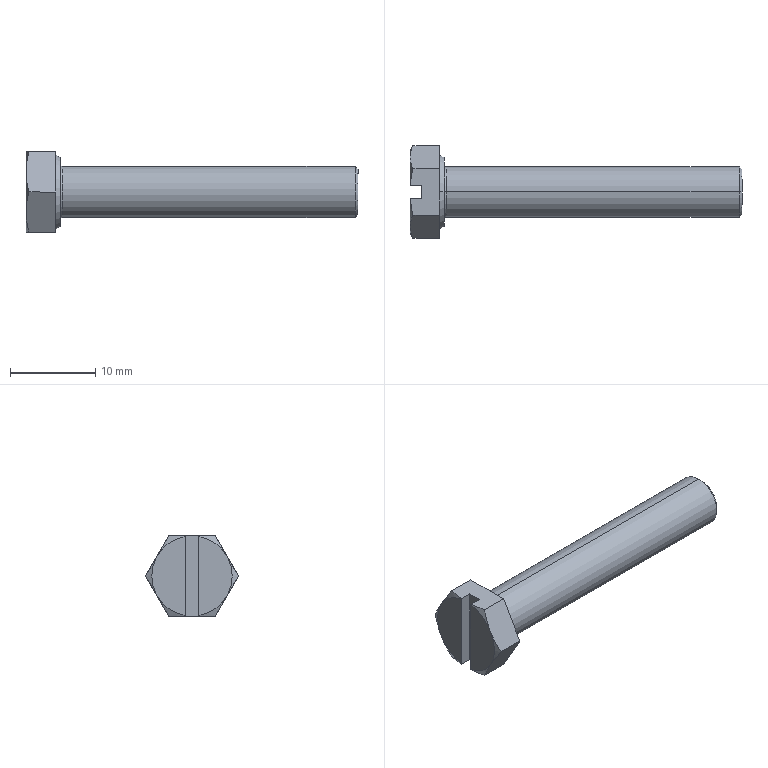Part | SolidWorks | features Cut 2, Chamfer 1, Extrusion 1, Fillet 1, LPattern 1, MoveCopyBody 1, RevCut 1, Revolution 1 | 1 solid | 24 faces | box 39 x 10.9 x 9.44 mm | volume 1265 mm3 | plane 14 | cone 6 | torus 2 | cylinder 2 | commonest cylinder face diameters 6 x2
STEP:
#1=CARTESIAN_POINT('',(28.65,0.,-9.517));
#2=VERTEX_POINT('',#1);
#3=CARTESIAN_POINT('',(28.65,0.,-4.183));
#4=VERTEX_POINT('',#3);
#5=CARTESIAN_POINT('',(28.65,0.,-6.85));
#6=DIRECTION('',(1.,0.,0.));
#7=DIRECTION('',(0.,0.,1.));
#8=AXIS2_PLACEMENT_3D('',#5,#6,#7);
#9=CIRCLE('',#8,2.667);
#10=EDGE_CURVE('',#2,#4,#9,.T.);
#11=ORIENTED_EDGE('',*,*,#10,.F.);
#12=CARTESIAN_POINT('',(28.317,0.,-9.85));
#13=VERTEX_POINT('',#12);
#14=CARTESIAN_POINT('',(28.317,0.,-9.85));
#15=DIRECTION('',(-0.7071,0.,-0.7071));
#16=VECTOR('',#15,1000.);
#17=LINE('',#14,#16);
#18=EDGE_CURVE('',#2,#13,#17,.T.);
#19=ORIENTED_EDGE('',*,*,#18,.T.);
#20=CARTESIAN_POINT('',(28.317,0.,-3.85));
#21=VERTEX_POINT('',#20);
#22=CARTESIAN_POINT('',(28.317,0.,-6.85));
#23=DIRECTION('',(-1.,0.,0.));
#24=DIRECTION('',(0.,0.,1.));
#25=AXIS2_PLACEMENT_3D('',#22,#23,#24);
#26=CIRCLE('',#25,3.);
#27=EDGE_CURVE('',#21,#13,#26,.T.);
#28=ORIENTED_EDGE('',*,*,#27,.F.);
#29=CARTESIAN_POINT('',(28.317,0.,-3.85));
#30=DIRECTION('',(-0.7071,0.,0.7071));
#31=VECTOR('',#30,1000.);
#32=LINE('',#29,#31);
#33=EDGE_CURVE('',#4,#21,#32,.T.);
#34=ORIENTED_EDGE('',*,*,#33,.F.);
#35=EDGE_LOOP('',(#11,#19,#28,#34));
#36=FACE_OUTER_BOUND('',#35,.T.);
#37=CARTESIAN_POINT('',(28.317,0.,-6.85));
#38=DIRECTION('',(-1.,0.,0.));
#39=DIRECTION('',(0.,0.,1.));
#40=AXIS2_PLACEMENT_3D('',#37,#38,#39);
#41=CONICAL_SURFACE('',#40,3.,0.7854);
#42=ADVANCED_FACE('',(#36),#41,.T.);
#43=CARTESIAN_POINT('',(-6.35,0.,-10.1));
#44=VERTEX_POINT('',#43);
#45=CARTESIAN_POINT('',(-6.35,0.,-3.6));
#46=VERTEX_POINT('',#45);
#47=CARTESIAN_POINT('',(-6.35,0.,-6.85));
#48=DIRECTION('',(-1.,0.,0.));
#49=DIRECTION('',(0.,0.,1.));
#50=AXIS2_PLACEMENT_3D('',#47,#48,#49);
#51=CIRCLE('',#50,3.25);
#52=EDGE_CURVE('',#44,#46,#51,.T.);
#53=ORIENTED_EDGE('',*,*,#52,.F.);
#54=CARTESIAN_POINT('',(-6.1,0.,-9.85));
#55=VERTEX_POINT('',#54);
#56=CARTESIAN_POINT('',(-6.1,0.,-10.1));
#57=DIRECTION('',(0.,1.,0.));
#58=DIRECTION('',(0.,0.,1.));
#59=AXIS2_PLACEMENT_3D('',#56,#57,#58);
#60=CIRCLE('',#59,0.25);
#61=EDGE_CURVE('',#44,#55,#60,.T.);
#62=ORIENTED_EDGE('',*,*,#61,.T.);
#63=CARTESIAN_POINT('',(-6.1,0.,-3.85));
#64=VERTEX_POINT('',#63);
#65=CARTESIAN_POINT('',(-6.1,0.,-6.85));
#66=DIRECTION('',(1.,0.,0.));
#67=DIRECTION('',(0.,0.,1.));
#68=AXIS2_PLACEMENT_3D('',#65,#66,#67);
#69=CIRCLE('',#68,3.);
#70=EDGE_CURVE('',#64,#55,#69,.T.);
#71=ORIENTED_EDGE('',*,*,#70,.F.);
#72=CARTESIAN_POINT('',(-6.1,0.,-3.6));
#73=DIRECTION('',(0.,-1.,0.));
#74=DIRECTION('',(0.,0.,-1.));
#75=AXIS2_PLACEMENT_3D('',#72,#73,#74);
#76=CIRCLE('',#75,0.25);
#77=EDGE_CURVE('',#46,#64,#76,.T.);
#78=ORIENTED_EDGE('',*,*,#77,.F.);
#79=EDGE_LOOP('',(#53,#62,#71,#78));
#80=FACE_OUTER_BOUND('',#79,.T.);
#81=CARTESIAN_POINT('',(-6.1,0.,-6.85));
#82=DIRECTION('',(-1.,0.,0.));
#83=DIRECTION('',(0.,0.,1.));
#84=AXIS2_PLACEMENT_3D('',#81,#82,#83);
#85=TOROIDAL_SURFACE('',#84,3.25,0.25);
#86=ADVANCED_FACE('',(#80),#85,.F.);
#87=CARTESIAN_POINT('',(-6.35,0.,-2.789));
#88=VERTEX_POINT('',#87);
#89=CARTESIAN_POINT('',(-6.35,0.,-10.911));
#90=VERTEX_POINT('',#89);
#91=CARTESIAN_POINT('',(-6.35,0.,-6.85));
#92=DIRECTION('',(-1.,0.,0.));
#93=DIRECTION('',(0.,0.,1.));
#94=AXIS2_PLACEMENT_3D('',#91,#92,#93);
#95=CIRCLE('',#94,4.061);
#96=EDGE_CURVE('',#88,#90,#95,.T.);
#97=ORIENTED_EDGE('',*,*,#96,.T.);
#98=CARTESIAN_POINT('',(-6.85,0.,-11.2));
#99=VERTEX_POINT('',#98);
#100=CARTESIAN_POINT('',(-6.35,0.,-10.911));
#101=DIRECTION('',(-0.866,0.,-0.5));
#102=VECTOR('',#101,1000.);
#103=LINE('',#100,#102);
#104=EDGE_CURVE('',#90,#99,#103,.T.);
#105=ORIENTED_EDGE('',*,*,#104,.T.);
#106=CARTESIAN_POINT('',(-6.85,0.,-2.5));
#107=VERTEX_POINT('',#106);
#108=CARTESIAN_POINT('',(-6.85,0.,-6.85));
#109=DIRECTION('',(1.,0.,0.));
#110=DIRECTION('',(0.,0.,1.));
#111=AXIS2_PLACEMENT_3D('',#108,#109,#110);
#112=CIRCLE('',#111,4.35);
#113=EDGE_CURVE('',#99,#107,#112,.T.);
#114=ORIENTED_EDGE('',*,*,#113,.T.);
#115=CARTESIAN_POINT('',(-6.35,0.,-2.789));
#116=DIRECTION('',(-0.866,0.,0.5));
#117=VECTOR('',#116,1000.);
#118=LINE('',#115,#117);
#119=EDGE_CURVE('',#88,#107,#118,.T.);
#120=ORIENTED_EDGE('',*,*,#119,.F.);
#121=EDGE_LOOP('',(#97,#105,#114,#120));
#122=FACE_OUTER_BOUND('',#121,.T.);
#123=CARTESIAN_POINT('',(-6.35,0.,-6.85));
#124=DIRECTION('',(-1.,0.,0.));
#125=DIRECTION('',(0.,0.,1.));
#126=AXIS2_PLACEMENT_3D('',#123,#124,#125);
#127=CONICAL_SURFACE('',#126,4.061,0.5236);
#128=ADVANCED_FACE('',(#122),#127,.T.);
#129=ORIENTED_EDGE('',*,*,#27,.T.);
#130=CARTESIAN_POINT('',(-6.85,0.,-9.85));
#131=DIRECTION('',(-1.,0.,0.));
#132=VECTOR('',#131,1000.);
#133=LINE('',#130,#132);
#134=EDGE_CURVE('',#13,#55,#133,.T.);
#135=ORIENTED_EDGE('',*,*,#134,.T.);
#136=CARTESIAN_POINT('',(-6.1,0.,-6.85));
#137=DIRECTION('',(1.,0.,0.));
#138=DIRECTION('',(0.,0.,1.));
#139=AXIS2_PLACEMENT_3D('',#136,#137,#138);
#140=CIRCLE('',#139,3.);
#141=EDGE_CURVE('',#55,#64,#140,.T.);
#142=ORIENTED_EDGE('',*,*,#141,.T.);
#143=CARTESIAN_POINT('',(-6.85,0.,-3.85));
#144=DIRECTION('',(-1.,0.,0.));
#145=VECTOR('',#144,1000.);
#146=LINE('',#143,#145);
#147=EDGE_CURVE('',#21,#64,#146,.T.);
#148=ORIENTED_EDGE('',*,*,#147,.F.);
#149=EDGE_LOOP('',(#129,#135,#142,#148));
#150=FACE_OUTER_BOUND('',#149,.T.);
#151=CARTESIAN_POINT('',(-6.85,0.,-6.85));
#152=DIRECTION('',(-1.,0.,0.));
#153=DIRECTION('',(0.,0.,1.));
#154=AXIS2_PLACEMENT_3D('',#151,#152,#153);
#155=CYLINDRICAL_SURFACE('',#154,3.);
#156=ADVANCED_FACE('',(#150),#155,.T.);
#157=CARTESIAN_POINT('',(-10.319,-0.8,-11.57));
#158=VERTEX_POINT('',#157);
#159=CARTESIAN_POINT('',(-10.35,-0.8,-11.501));
#160=VERTEX_POINT('',#159);
#161=CARTESIAN_POINT('',(-10.319,-0.8,-11.57));
#162=CARTESIAN_POINT('',(-10.329,-0.8,-11.547));
#163=CARTESIAN_POINT('',(-10.34,-0.8,-11.524));
#164=CARTESIAN_POINT('',(-10.35,-0.8,-11.501));
#165=B_SPLINE_CURVE_WITH_KNOTS('',3,(#161,#162,#163,#164),.UNSPECIFIED.,.F.,.F.,(4,4),(0.006283,0.006358),.UNSPECIFIED.);
#166=EDGE_CURVE('',#158,#160,#165,.T.);
#167=ORIENTED_EDGE('',*,*,#166,.F.);
#168=CARTESIAN_POINT('',(-10.009,-2.725,-11.57));
#169=VERTEX_POINT('',#168);
#170=CARTESIAN_POINT('',(-10.319,-0.8,-11.57));
#171=CARTESIAN_POINT('',(-10.293,-1.122,-11.57));
#172=CARTESIAN_POINT('',(-10.254,-1.444,-11.57));
#173=CARTESIAN_POINT('',(-10.149,-2.086,-11.57));
#174=CARTESIAN_POINT('',(-10.083,-2.408,-11.57));
#175=CARTESIAN_POINT('',(-10.009,-2.725,-11.57));
#176=B_SPLINE_CURVE_WITH_KNOTS('',3,(#170,#171,#172,#173,#174,#175),.UNSPECIFIED.,.F.,.F.,(4,2,4),(0.01518,0.01614,0.0171),.UNSPECIFIED.);
#177=EDGE_CURVE('',#158,#169,#176,.T.);
#178=ORIENTED_EDGE('',*,*,#177,.T.);
#179=CARTESIAN_POINT('',(-10.009,-5.45,-6.85));
#180=VERTEX_POINT('',#179);
#181=CARTESIAN_POINT('',(-10.009,-2.725,-11.57));
#182=CARTESIAN_POINT('',(-10.219,-3.174,-10.792));
#183=CARTESIAN_POINT('',(-10.349,-3.626,-10.01));
#184=CARTESIAN_POINT('',(-10.35,-4.309,-8.826));
#185=CARTESIAN_POINT('',(-10.32,-4.539,-8.428));
#186=CARTESIAN_POINT('',(-10.201,-4.998,-7.633));
#187=CARTESIAN_POINT('',(-10.115,-5.225,-7.24));
#188=CARTESIAN_POINT('',(-10.009,-5.45,-6.85));
#189=B_SPLINE_CURVE_WITH_KNOTS('',3,(#181,#182,#183,#184,#185,#186,#187,#188),.UNSPECIFIED.,.F.,.F.,(4,2,2,4),(0.000000234,0.00273,0.004094,0.005459),.UNSPECIFIED.);
#190=EDGE_CURVE('',#169,#180,#189,.T.);
#191=ORIENTED_EDGE('',*,*,#190,.T.);
#192=CARTESIAN_POINT('',(-10.009,-2.725,-2.13));
#193=VERTEX_POINT('',#192);
#194=CARTESIAN_POINT('',(-10.009,-5.45,-6.85));
#195=CARTESIAN_POINT('',(-10.219,-5.001,-6.072));
#196=CARTESIAN_POINT('',(-10.349,-4.549,-5.29));
#197=CARTESIAN_POINT('',(-10.35,-3.866,-4.106));
#198=CARTESIAN_POINT('',(-10.32,-3.636,-3.708));
#199=CARTESIAN_POINT('',(-10.201,-3.177,-2.914));
#200=CARTESIAN_POINT('',(-10.115,-2.95,-2.52));
#201=CARTESIAN_POINT('',(-10.009,-2.725,-2.13));
#202=B_SPLINE_CURVE_WITH_KNOTS('',3,(#194,#195,#196,#197,#198,#199,#200,#201),.UNSPECIFIED.,.F.,.F.,(4,2,2,4),(0.000000234,0.00273,0.004094,0.005459),.UNSPECIFIED.);
#203=EDGE_CURVE('',#180,#193,#202,.T.);
#204=ORIENTED_EDGE('',*,*,#203,.T.);
#205=CARTESIAN_POINT('',(-10.319,-0.8,-2.13));
#206=VERTEX_POINT('',#205);
#207=CARTESIAN_POINT('',(-10.009,-2.725,-2.13));
#208=CARTESIAN_POINT('',(-10.083,-2.408,-2.13));
#209=CARTESIAN_POINT('',(-10.149,-2.086,-2.13));
#210=CARTESIAN_POINT('',(-10.254,-1.444,-2.13));
#211=CARTESIAN_POINT('',(-10.293,-1.122,-2.13));
#212=CARTESIAN_POINT('',(-10.319,-0.8,-2.13));
#213=B_SPLINE_CURVE_WITH_KNOTS('',3,(#207,#208,#209,#210,#211,#212),.UNSPECIFIED.,.F.,.F.,(4,2,4),(0.004915,0.00589,0.006864),.UNSPECIFIED.);
#214=EDGE_CURVE('',#193,#206,#213,.T.);
#215=ORIENTED_EDGE('',*,*,#214,.T.);
#216=CARTESIAN_POINT('',(-10.35,-0.8,-2.199));
#217=VERTEX_POINT('',#216);
#218=CARTESIAN_POINT('',(-10.35,-0.8,-2.199));
#219=CARTESIAN_POINT('',(-10.34,-0.8,-2.176));
#220=CARTESIAN_POINT('',(-10.329,-0.8,-2.153));
#221=CARTESIAN_POINT('',(-10.319,-0.8,-2.13));
#222=B_SPLINE_CURVE_WITH_KNOTS('',3,(#218,#219,#220,#221),.UNSPECIFIED.,.F.,.F.,(4,4),(0.01639,0.01646),.UNSPECIFIED.);
#223=EDGE_CURVE('',#217,#206,#222,.T.);
#224=ORIENTED_EDGE('',*,*,#223,.F.);
#225=CARTESIAN_POINT('',(-10.35,0.,-6.85));
#226=DIRECTION('',(-1.,0.,0.));
#227=DIRECTION('',(0.,0.,1.));
#228=AXIS2_PLACEMENT_3D('',#225,#226,#227);
#229=CIRCLE('',#228,4.72);
#230=EDGE_CURVE('',#160,#217,#229,.T.);
#231=ORIENTED_EDGE('',*,*,#230,.F.);
#232=EDGE_LOOP('',(#167,#178,#191,#204,#215,#224,#231));
#233=FACE_OUTER_BOUND('',#232,.T.);
#234=CARTESIAN_POINT('',(-10.35,0.,-6.85));
#235=DIRECTION('',(1.,0.,0.));
#236=DIRECTION('',(0.,0.,1.));
#237=AXIS2_PLACEMENT_3D('',#234,#235,#236);
#238=CONICAL_SURFACE('',#237,4.72,1.134);
#239=ADVANCED_FACE('',(#233),#238,.T.);
#240=CARTESIAN_POINT('',(-10.35,-0.8,-11.57));
#241=DIRECTION('',(0.,0.,1.));
#242=VECTOR('',#241,1000.);
#243=LINE('',#240,#242);
#244=EDGE_CURVE('',#160,#217,#243,.T.);
#245=ORIENTED_EDGE('',*,*,#244,.F.);
#246=ORIENTED_EDGE('',*,*,#230,.T.);
#247=EDGE_LOOP('',(#245,#246));
#248=FACE_OUTER_BOUND('',#247,.T.);
#249=CARTESIAN_POINT('',(-10.35,8.175,-11.57));
#250=DIRECTION('',(-1.,0.,0.));
#251=DIRECTION('',(0.,0.,1.));
#252=AXIS2_PLACEMENT_3D('',#249,#250,#251);
#253=PLANE('',#252);
#254=ADVANCED_FACE('',(#248),#253,.T.);
#255=CARTESIAN_POINT('',(-6.85,2.725,-2.13));
#256=VERTEX_POINT('',#255);
#257=CARTESIAN_POINT('',(-6.85,5.45,-6.85));
#258=VERTEX_POINT('',#257);
#259=CARTESIAN_POINT('',(-6.85,2.725,-2.13));
#260=DIRECTION('',(0.,0.5,-0.866));
#261=VECTOR('',#260,1000.);
#262=LINE('',#259,#261);
#263=EDGE_CURVE('',#256,#258,#262,.T.);
#264=ORIENTED_EDGE('',*,*,#263,.F.);
#265=CARTESIAN_POINT('',(-6.85,-2.725,-2.13));
#266=VERTEX_POINT('',#265);
#267=CARTESIAN_POINT('',(-6.85,-2.725,-2.13));
#268=DIRECTION('',(0.,1.,0.));
#269=VECTOR('',#268,1000.);
#270=LINE('',#267,#269);
#271=EDGE_CURVE('',#266,#256,#270,.T.);
#272=ORIENTED_EDGE('',*,*,#271,.F.);
#273=CARTESIAN_POINT('',(-6.85,-5.45,-6.85));
#274=VERTEX_POINT('',#273);
#275=CARTESIAN_POINT('',(-6.85,-5.45,-6.85));
#276=DIRECTION('',(0.,0.5,0.866));
#277=VECTOR('',#276,1000.);
#278=LINE('',#275,#277);
#279=EDGE_CURVE('',#274,#266,#278,.T.);
#280=ORIENTED_EDGE('',*,*,#279,.F.);
#281=CARTESIAN_POINT('',(-6.85,-2.725,-11.57));
#282=VERTEX_POINT('',#281);
#283=CARTESIAN_POINT('',(-6.85,-2.725,-11.57));
#284=DIRECTION('',(0.,-0.5,0.866));
#285=VECTOR('',#284,1000.);
#286=LINE('',#283,#285);
#287=EDGE_CURVE('',#282,#274,#286,.T.);
#288=ORIENTED_EDGE('',*,*,#287,.F.);
#289=CARTESIAN_POINT('',(-6.85,2.725,-11.57));
#290=VERTEX_POINT('',#289);
#291=CARTESIAN_POINT('',(-6.85,2.725,-11.57));
#292=DIRECTION('',(0.,-1.,0.));
#293=VECTOR('',#292,1000.);
#294=LINE('',#291,#293);
#295=EDGE_CURVE('',#290,#282,#294,.T.);
#296=ORIENTED_EDGE('',*,*,#295,.F.);
#297=CARTESIAN_POINT('',(-6.85,5.45,-6.85));
#298=DIRECTION('',(0.,-0.5,-0.866));
#299=VECTOR('',#298,1000.);
#300=LINE('',#297,#299);
#301=EDGE_CURVE('',#258,#290,#300,.T.);
#302=ORIENTED_EDGE('',*,*,#301,.F.);
#303=EDGE_LOOP('',(#264,#272,#280,#288,#296,#302));
#304=FACE_OUTER_BOUND('',#303,.T.);
#305=CARTESIAN_POINT('',(-6.85,0.,-6.85));
#306=DIRECTION('',(1.,0.,0.));
#307=DIRECTION('',(0.,0.,1.));
#308=AXIS2_PLACEMENT_3D('',#305,#306,#307);
#309=CIRCLE('',#308,4.35);
#310=EDGE_CURVE('',#107,#99,#309,.T.);
#311=ORIENTED_EDGE('',*,*,#310,.F.);
#312=ORIENTED_EDGE('',*,*,#113,.F.);
#313=EDGE_LOOP('',(#311,#312));
#314=FACE_BOUND('',#313,.T.);
#315=CARTESIAN_POINT('',(-6.85,8.175,-11.57));
#316=DIRECTION('',(-1.,0.,0.));
#317=DIRECTION('',(0.,0.,1.));
#318=AXIS2_PLACEMENT_3D('',#315,#316,#317);
#319=PLANE('',#318);
#320=ADVANCED_FACE('',(#304,#314),#319,.F.);
#321=CARTESIAN_POINT('',(-10.009,2.725,-2.13));
#322=VERTEX_POINT('',#321);
#323=CARTESIAN_POINT('',(-10.009,5.45,-6.85));
#324=VERTEX_POINT('',#323);
#325=CARTESIAN_POINT('',(-10.009,2.725,-2.13));
#326=CARTESIAN_POINT('',(-10.219,3.174,-2.908));
#327=CARTESIAN_POINT('',(-10.349,3.626,-3.69));
#328=CARTESIAN_POINT('',(-10.35,4.309,-4.874));
#329=CARTESIAN_POINT('',(-10.32,4.539,-5.272));
#330=CARTESIAN_POINT('',(-10.201,4.998,-6.067));
#331=CARTESIAN_POINT('',(-10.115,5.225,-6.46));
#332=CARTESIAN_POINT('',(-10.009,5.45,-6.85));
#333=B_SPLINE_CURVE_WITH_KNOTS('',3,(#325,#326,#327,#328,#329,#330,#331,#332),.UNSPECIFIED.,.F.,.F.,(4,2,2,4),(0.000000234,0.00273,0.004094,0.005459),.UNSPECIFIED.);
#334=EDGE_CURVE('',#322,#324,#333,.T.);
#335=ORIENTED_EDGE('',*,*,#334,.F.);
#336=CARTESIAN_POINT('',(-10.35,2.725,-2.13));
#337=DIRECTION('',(1.,0.,0.));
#338=VECTOR('',#337,1000.);
#339=LINE('',#336,#338);
#340=EDGE_CURVE('',#322,#256,#339,.T.);
#341=ORIENTED_EDGE('',*,*,#340,.T.);
#342=ORIENTED_EDGE('',*,*,#263,.T.);
#343=CARTESIAN_POINT('',(-10.35,5.45,-6.85));
#344=DIRECTION('',(1.,0.,0.));
#345=VECTOR('',#344,1000.);
#346=LINE('',#343,#345);
#347=EDGE_CURVE('',#324,#258,#346,.T.);
#348=ORIENTED_EDGE('',*,*,#347,.F.);
#349=EDGE_LOOP('',(#335,#341,#342,#348));
#350=FACE_OUTER_BOUND('',#349,.T.);
#351=CARTESIAN_POINT('',(-10.35,2.725,-2.13));
#352=DIRECTION('',(0.,-0.866,-0.5));
#353=DIRECTION('',(0.,-0.5,0.866));
#354=AXIS2_PLACEMENT_3D('',#351,#352,#353);
#355=PLANE('',#354);
#356=ADVANCED_FACE('',(#350),#355,.F.);
#357=CARTESIAN_POINT('',(-10.009,2.725,-11.57));
#358=VERTEX_POINT('',#357);
#359=CARTESIAN_POINT('',(-10.009,5.45,-6.85));
#360=CARTESIAN_POINT('',(-10.219,5.001,-7.628));
#361=CARTESIAN_POINT('',(-10.349,4.549,-8.41));
#362=CARTESIAN_POINT('',(-10.35,3.866,-9.594));
#363=CARTESIAN_POINT('',(-10.32,3.636,-9.992));
#364=CARTESIAN_POINT('',(-10.201,3.177,-10.786));
#365=CARTESIAN_POINT('',(-10.115,2.95,-11.18));
#366=CARTESIAN_POINT('',(-10.009,2.725,-11.57));
#367=B_SPLINE_CURVE_WITH_KNOTS('',3,(#359,#360,#361,#362,#363,#364,#365,#366),.UNSPECIFIED.,.F.,.F.,(4,2,2,4),(0.000000234,0.00273,0.004094,0.005459),.UNSPECIFIED.);
#368=EDGE_CURVE('',#324,#358,#367,.T.);
#369=ORIENTED_EDGE('',*,*,#368,.F.);
#370=ORIENTED_EDGE('',*,*,#347,.T.);
#371=ORIENTED_EDGE('',*,*,#301,.T.);
#372=CARTESIAN_POINT('',(-10.35,2.725,-11.57));
#373=DIRECTION('',(1.,0.,0.));
#374=VECTOR('',#373,1000.);
#375=LINE('',#372,#374);
#376=EDGE_CURVE('',#358,#290,#375,.T.);
#377=ORIENTED_EDGE('',*,*,#376,.F.);
#378=EDGE_LOOP('',(#369,#370,#371,#377));
#379=FACE_OUTER_BOUND('',#378,.T.);
#380=CARTESIAN_POINT('',(-10.35,5.45,-6.85));
#381=DIRECTION('',(0.,-0.866,0.5));
#382=DIRECTION('',(0.,0.5,0.866));
#383=AXIS2_PLACEMENT_3D('',#380,#381,#382);
#384=PLANE('',#383);
#385=ADVANCED_FACE('',(#379),#384,.F.);
#386=ORIENTED_EDGE('',*,*,#177,.F.);
#387=CARTESIAN_POINT('',(-8.95,-0.8,-11.57));
#388=VERTEX_POINT('',#387);
#389=CARTESIAN_POINT('',(-8.95,-0.8,-11.57));
#390=DIRECTION('',(-1.,0.,0.));
#391=VECTOR('',#390,1000.);
#392=LINE('',#389,#391);
#393=EDGE_CURVE('',#388,#158,#392,.T.);
#394=ORIENTED_EDGE('',*,*,#393,.F.);
#395=CARTESIAN_POINT('',(-8.95,0.8,-11.57));
#396=VERTEX_POINT('',#395);
#397=CARTESIAN_POINT('',(-8.95,0.8,-11.57));
#398=DIRECTION('',(0.,-1.,0.));
#399=VECTOR('',#398,1000.);
#400=LINE('',#397,#399);
#401=EDGE_CURVE('',#396,#388,#400,.T.);
#402=ORIENTED_EDGE('',*,*,#401,.F.);
#403=CARTESIAN_POINT('',(-10.319,0.8,-11.57));
#404=VERTEX_POINT('',#403);
#405=CARTESIAN_POINT('',(-8.95,0.8,-11.57));
#406=DIRECTION('',(-1.,0.,0.));
#407=VECTOR('',#406,1000.);
#408=LINE('',#405,#407);
#409=EDGE_CURVE('',#396,#404,#408,.T.);
#410=ORIENTED_EDGE('',*,*,#409,.T.);
#411=CARTESIAN_POINT('',(-10.009,2.725,-11.57));
#412=CARTESIAN_POINT('',(-10.083,2.41,-11.57));
#413=CARTESIAN_POINT('',(-10.147,2.093,-11.57));
#414=CARTESIAN_POINT('',(-10.253,1.449,-11.57));
#415=CARTESIAN_POINT('',(-10.293,1.123,-11.57));
#416=CARTESIAN_POINT('',(-10.319,0.8,-11.57));
#417=B_SPLINE_CURVE_WITH_KNOTS('',3,(#411,#412,#413,#414,#415,#416),.UNSPECIFIED.,.F.,.F.,(4,2,4),(0.01167,0.01263,0.01359),.UNSPECIFIED.);
#418=EDGE_CURVE('',#358,#404,#417,.T.);
#419=ORIENTED_EDGE('',*,*,#418,.F.);
#420=ORIENTED_EDGE('',*,*,#376,.T.);
#421=ORIENTED_EDGE('',*,*,#295,.T.);
#422=CARTESIAN_POINT('',(-10.35,-2.725,-11.57));
#423=DIRECTION('',(1.,0.,0.));
#424=VECTOR('',#423,1000.);
#425=LINE('',#422,#424);
#426=EDGE_CURVE('',#169,#282,#425,.T.);
#427=ORIENTED_EDGE('',*,*,#426,.F.);
#428=EDGE_LOOP('',(#386,#394,#402,#410,#419,#420,#421,#427));
#429=FACE_OUTER_BOUND('',#428,.T.);
#430=CARTESIAN_POINT('',(-10.35,2.725,-11.57));
#431=DIRECTION('',(0.,0.,1.));
#432=DIRECTION('',(0.,1.,0.));
#433=AXIS2_PLACEMENT_3D('',#430,#431,#432);
#434=PLANE('',#433);
#435=ADVANCED_FACE('',(#429),#434,.F.);
#436=ORIENTED_EDGE('',*,*,#190,.F.);
#437=ORIENTED_EDGE('',*,*,#426,.T.);
#438=ORIENTED_EDGE('',*,*,#287,.T.);
#439=CARTESIAN_POINT('',(-10.35,-5.45,-6.85));
#440=DIRECTION('',(1.,0.,0.));
#441=VECTOR('',#440,1000.);
#442=LINE('',#439,#441);
#443=EDGE_CURVE('',#180,#274,#442,.T.);
#444=ORIENTED_EDGE('',*,*,#443,.F.);
#445=EDGE_LOOP('',(#436,#437,#438,#444));
#446=FACE_OUTER_BOUND('',#445,.T.);
#447=CARTESIAN_POINT('',(-10.35,-2.725,-11.57));
#448=DIRECTION('',(0.,0.866,0.5));
#449=DIRECTION('',(0.,0.5,-0.866));
#450=AXIS2_PLACEMENT_3D('',#447,#448,#449);
#451=PLANE('',#450);
#452=ADVANCED_FACE('',(#446),#451,.F.);
#453=ORIENTED_EDGE('',*,*,#203,.F.);
#454=ORIENTED_EDGE('',*,*,#443,.T.);
#455=ORIENTED_EDGE('',*,*,#279,.T.);
#456=CARTESIAN_POINT('',(-10.35,-2.725,-2.13));
#457=DIRECTION('',(1.,0.,0.));
#458=VECTOR('',#457,1000.);
#459=LINE('',#456,#458);
#460=EDGE_CURVE('',#193,#266,#459,.T.);
#461=ORIENTED_EDGE('',*,*,#460,.F.);
#462=EDGE_LOOP('',(#453,#454,#455,#461));
#463=FACE_OUTER_BOUND('',#462,.T.);
#464=CARTESIAN_POINT('',(-10.35,-5.45,-6.85));
#465=DIRECTION('',(0.,0.866,-0.5));
#466=DIRECTION('',(0.,-0.5,-0.866));
#467=AXIS2_PLACEMENT_3D('',#464,#465,#466);
#468=PLANE('',#467);
#469=ADVANCED_FACE('',(#463),#468,.F.);
#470=CARTESIAN_POINT('',(-8.95,-0.8,-2.13));
#471=VERTEX_POINT('',#470);
#472=CARTESIAN_POINT('',(-8.95,0.8,-2.13));
#473=VERTEX_POINT('',#472);
#474=CARTESIAN_POINT('',(-8.95,-0.8,-2.13));
#475=DIRECTION('',(0.,1.,0.));
#476=VECTOR('',#475,1000.);
#477=LINE('',#474,#476);
#478=EDGE_CURVE('',#471,#473,#477,.T.);
#479=ORIENTED_EDGE('',*,*,#478,.F.);
#480=CARTESIAN_POINT('',(-8.95,-0.8,-2.13));
#481=DIRECTION('',(-1.,0.,0.));
#482=VECTOR('',#481,1000.);
#483=LINE('',#480,#482);
#484=EDGE_CURVE('',#471,#206,#483,.T.);
#485=ORIENTED_EDGE('',*,*,#484,.T.);
#486=ORIENTED_EDGE('',*,*,#214,.F.);
#487=ORIENTED_EDGE('',*,*,#460,.T.);
#488=ORIENTED_EDGE('',*,*,#271,.T.);
#489=ORIENTED_EDGE('',*,*,#340,.F.);
#490=CARTESIAN_POINT('',(-10.319,0.8,-2.13));
#491=VERTEX_POINT('',#490);
#492=CARTESIAN_POINT('',(-10.319,0.8,-2.13));
#493=CARTESIAN_POINT('',(-10.293,1.123,-2.13));
#494=CARTESIAN_POINT('',(-10.253,1.449,-2.13));
#495=CARTESIAN_POINT('',(-10.147,2.093,-2.13));
#496=CARTESIAN_POINT('',(-10.083,2.41,-2.13));
#497=CARTESIAN_POINT('',(-10.009,2.725,-2.13));
#498=B_SPLINE_CURVE_WITH_KNOTS('',3,(#492,#493,#494,#495,#496,#497),.UNSPECIFIED.,.F.,.F.,(4,2,4),(0.008474,0.009449,0.01042),.UNSPECIFIED.);
#499=EDGE_CURVE('',#491,#322,#498,.T.);
#500=ORIENTED_EDGE('',*,*,#499,.F.);
#501=CARTESIAN_POINT('',(-8.95,0.8,-2.13));
#502=DIRECTION('',(-1.,0.,0.));
#503=VECTOR('',#502,1000.);
#504=LINE('',#501,#503);
#505=EDGE_CURVE('',#473,#491,#504,.T.);
#506=ORIENTED_EDGE('',*,*,#505,.F.);
#507=EDGE_LOOP('',(#479,#485,#486,#487,#488,#489,#500,#506));
#508=FACE_OUTER_BOUND('',#507,.T.);
#509=CARTESIAN_POINT('',(-10.35,-2.725,-2.13));
#510=DIRECTION('',(0.,0.,-1.));
#511=DIRECTION('',(0.,-1.,0.));
#512=AXIS2_PLACEMENT_3D('',#509,#510,#511);
#513=PLANE('',#512);
#514=ADVANCED_FACE('',(#508),#513,.F.);
#515=CARTESIAN_POINT('',(-10.35,0.8,-2.199));
#516=VERTEX_POINT('',#515);
#517=CARTESIAN_POINT('',(-10.319,0.8,-2.13));
#518=CARTESIAN_POINT('',(-10.329,0.8,-2.153));
#519=CARTESIAN_POINT('',(-10.34,0.8,-2.176));
#520=CARTESIAN_POINT('',(-10.35,0.8,-2.199));
#521=B_SPLINE_CURVE_WITH_KNOTS('',3,(#517,#518,#519,#520),.UNSPECIFIED.,.F.,.F.,(4,4),(0.006283,0.006358),.UNSPECIFIED.);
#522=EDGE_CURVE('',#491,#516,#521,.T.);
#523=ORIENTED_EDGE('',*,*,#522,.F.);
#524=ORIENTED_EDGE('',*,*,#499,.T.);
#525=ORIENTED_EDGE('',*,*,#334,.T.);
#526=ORIENTED_EDGE('',*,*,#368,.T.);
#527=ORIENTED_EDGE('',*,*,#418,.T.);
#528=CARTESIAN_POINT('',(-10.35,0.8,-11.501));
#529=VERTEX_POINT('',#528);
#530=CARTESIAN_POINT('',(-10.35,0.8,-11.501));
#531=CARTESIAN_POINT('',(-10.34,0.8,-11.524));
#532=CARTESIAN_POINT('',(-10.329,0.8,-11.547));
#533=CARTESIAN_POINT('',(-10.319,0.8,-11.57));
#534=B_SPLINE_CURVE_WITH_KNOTS('',3,(#530,#531,#532,#533),.UNSPECIFIED.,.F.,.F.,(4,4),(0.01639,0.01646),.UNSPECIFIED.);
#535=EDGE_CURVE('',#529,#404,#534,.T.);
#536=ORIENTED_EDGE('',*,*,#535,.F.);
#537=CARTESIAN_POINT('',(-10.35,0.,-6.85));
#538=DIRECTION('',(-1.,0.,0.));
#539=DIRECTION('',(0.,0.,1.));
#540=AXIS2_PLACEMENT_3D('',#537,#538,#539);
#541=CIRCLE('',#540,4.72);
#542=EDGE_CURVE('',#516,#529,#541,.T.);
#543=ORIENTED_EDGE('',*,*,#542,.F.);
#544=EDGE_LOOP('',(#523,#524,#525,#526,#527,#536,#543));
#545=FACE_OUTER_BOUND('',#544,.T.);
#546=CARTESIAN_POINT('',(-10.35,0.,-6.85));
#547=DIRECTION('',(1.,0.,0.));
#548=DIRECTION('',(0.,0.,1.));
#549=AXIS2_PLACEMENT_3D('',#546,#547,#548);
#550=CONICAL_SURFACE('',#549,4.72,1.134);
#551=ADVANCED_FACE('',(#545),#550,.T.);
#552=CARTESIAN_POINT('',(-10.35,0.8,-11.57));
#553=DIRECTION('',(0.,0.,-1.));
#554=VECTOR('',#553,1000.);
#555=LINE('',#552,#554);
#556=EDGE_CURVE('',#516,#529,#555,.T.);
#557=ORIENTED_EDGE('',*,*,#556,.F.);
#558=ORIENTED_EDGE('',*,*,#542,.T.);
#559=EDGE_LOOP('',(#557,#558));
#560=FACE_OUTER_BOUND('',#559,.T.);
#561=CARTESIAN_POINT('',(-10.35,8.175,-11.57));
#562=DIRECTION('',(-1.,0.,0.));
#563=DIRECTION('',(0.,0.,1.));
#564=AXIS2_PLACEMENT_3D('',#561,#562,#563);
#565=PLANE('',#564);
#566=ADVANCED_FACE('',(#560),#565,.T.);
#567=CARTESIAN_POINT('',(-6.35,0.,-6.85));
#568=DIRECTION('',(-1.,0.,0.));
#569=DIRECTION('',(0.,0.,1.));
#570=AXIS2_PLACEMENT_3D('',#567,#568,#569);
#571=CIRCLE('',#570,3.25);
#572=EDGE_CURVE('',#46,#44,#571,.T.);
#573=ORIENTED_EDGE('',*,*,#572,.T.);
#574=ORIENTED_EDGE('',*,*,#52,.T.);
#575=EDGE_LOOP('',(#573,#574));
#576=FACE_BOUND('',#575,.T.);
#577=ORIENTED_EDGE('',*,*,#96,.F.);
#578=CARTESIAN_POINT('',(-6.35,0.,-6.85));
#579=DIRECTION('',(-1.,0.,0.));
#580=DIRECTION('',(0.,0.,1.));
#581=AXIS2_PLACEMENT_3D('',#578,#579,#580);
#582=CIRCLE('',#581,4.061);
#583=EDGE_CURVE('',#90,#88,#582,.T.);
#584=ORIENTED_EDGE('',*,*,#583,.F.);
#585=EDGE_LOOP('',(#577,#584));
#586=FACE_OUTER_BOUND('',#585,.T.);
#587=CARTESIAN_POINT('',(-6.35,3.,-6.85));
#588=DIRECTION('',(-1.,0.,0.));
#589=DIRECTION('',(0.,0.,1.));
#590=AXIS2_PLACEMENT_3D('',#587,#588,#589);
#591=PLANE('',#590);
#592=ADVANCED_FACE('',(#576,#586),#591,.F.);
#593=ORIENTED_EDGE('',*,*,#134,.F.);
#594=CARTESIAN_POINT('',(28.317,0.,-6.85));
#595=DIRECTION('',(-1.,0.,0.));
#596=DIRECTION('',(0.,0.,1.));
#597=AXIS2_PLACEMENT_3D('',#594,#595,#596);
#598=CIRCLE('',#597,3.);
#599=EDGE_CURVE('',#13,#21,#598,.T.);
#600=ORIENTED_EDGE('',*,*,#599,.T.);
#601=ORIENTED_EDGE('',*,*,#147,.T.);
#602=ORIENTED_EDGE('',*,*,#70,.T.);
#603=EDGE_LOOP('',(#593,#600,#601,#602));
#604=FACE_OUTER_BOUND('',#603,.T.);
#605=CARTESIAN_POINT('',(-6.85,0.,-6.85));
#606=DIRECTION('',(-1.,0.,0.));
#607=DIRECTION('',(0.,0.,1.));
#608=AXIS2_PLACEMENT_3D('',#605,#606,#607);
#609=CYLINDRICAL_SURFACE('',#608,3.);
#610=ADVANCED_FACE('',(#604),#609,.T.);
#611=CARTESIAN_POINT('',(28.65,0.,-6.85));
#612=DIRECTION('',(1.,0.,0.));
#613=DIRECTION('',(0.,0.,1.));
#614=AXIS2_PLACEMENT_3D('',#611,#612,#613);
#615=CIRCLE('',#614,2.667);
#616=EDGE_CURVE('',#4,#2,#615,.T.);
#617=ORIENTED_EDGE('',*,*,#616,.T.);
#618=ORIENTED_EDGE('',*,*,#10,.T.);
#619=EDGE_LOOP('',(#617,#618));
#620=FACE_OUTER_BOUND('',#619,.T.);
#621=CARTESIAN_POINT('',(28.65,3.,-6.85));
#622=DIRECTION('',(-1.,0.,0.));
#623=DIRECTION('',(0.,0.,1.));
#624=AXIS2_PLACEMENT_3D('',#621,#622,#623);
#625=PLANE('',#624);
#626=ADVANCED_FACE('',(#620),#625,.F.);
#627=ORIENTED_EDGE('',*,*,#104,.F.);
#628=ORIENTED_EDGE('',*,*,#583,.T.);
#629=ORIENTED_EDGE('',*,*,#119,.T.);
#630=ORIENTED_EDGE('',*,*,#310,.T.);
#631=EDGE_LOOP('',(#627,#628,#629,#630));
#632=FACE_OUTER_BOUND('',#631,.T.);
#633=CARTESIAN_POINT('',(-6.35,0.,-6.85));
#634=DIRECTION('',(-1.,0.,0.));
#635=DIRECTION('',(0.,0.,1.));
#636=AXIS2_PLACEMENT_3D('',#633,#634,#635);
#637=CONICAL_SURFACE('',#636,4.061,0.5236);
#638=ADVANCED_FACE('',(#632),#637,.T.);
#639=ORIENTED_EDGE('',*,*,#61,.F.);
#640=ORIENTED_EDGE('',*,*,#572,.F.);
#641=ORIENTED_EDGE('',*,*,#77,.T.);
#642=ORIENTED_EDGE('',*,*,#141,.F.);
#643=EDGE_LOOP('',(#639,#640,#641,#642));
#644=FACE_OUTER_BOUND('',#643,.T.);
#645=CARTESIAN_POINT('',(-6.1,0.,-6.85));
#646=DIRECTION('',(-1.,0.,0.));
#647=DIRECTION('',(0.,0.,1.));
#648=AXIS2_PLACEMENT_3D('',#645,#646,#647);
#649=TOROIDAL_SURFACE('',#648,3.25,0.25);
#650=ADVANCED_FACE('',(#644),#649,.F.);
#651=ORIENTED_EDGE('',*,*,#18,.F.);
#652=ORIENTED_EDGE('',*,*,#616,.F.);
#653=ORIENTED_EDGE('',*,*,#33,.T.);
#654=ORIENTED_EDGE('',*,*,#599,.F.);
#655=EDGE_LOOP('',(#651,#652,#653,#654));
#656=FACE_OUTER_BOUND('',#655,.T.);
#657=CARTESIAN_POINT('',(28.317,0.,-6.85));
#658=DIRECTION('',(-1.,0.,0.));
#659=DIRECTION('',(0.,0.,1.));
#660=AXIS2_PLACEMENT_3D('',#657,#658,#659);
#661=CONICAL_SURFACE('',#660,3.,0.7854);
#662=ADVANCED_FACE('',(#656),#661,.T.);
#663=ORIENTED_EDGE('',*,*,#166,.T.);
#664=ORIENTED_EDGE('',*,*,#244,.T.);
#665=ORIENTED_EDGE('',*,*,#223,.T.);
#666=ORIENTED_EDGE('',*,*,#484,.F.);
#667=CARTESIAN_POINT('',(-8.95,-0.8,-11.57));
#668=DIRECTION('',(0.,0.,1.));
#669=VECTOR('',#668,1000.);
#670=LINE('',#667,#669);
#671=EDGE_CURVE('',#388,#471,#670,.T.);
#672=ORIENTED_EDGE('',*,*,#671,.F.);
#673=ORIENTED_EDGE('',*,*,#393,.T.);
#674=EDGE_LOOP('',(#663,#664,#665,#666,#672,#673));
#675=FACE_OUTER_BOUND('',#674,.T.);
#676=CARTESIAN_POINT('',(-8.95,-0.8,-11.57));
#677=DIRECTION('',(0.,-1.,0.));
#678=DIRECTION('',(0.,0.,1.));
#679=AXIS2_PLACEMENT_3D('',#676,#677,#678);
#680=PLANE('',#679);
#681=ADVANCED_FACE('',(#675),#680,.F.);
#682=ORIENTED_EDGE('',*,*,#522,.T.);
#683=ORIENTED_EDGE('',*,*,#556,.T.);
#684=ORIENTED_EDGE('',*,*,#535,.T.);
#685=ORIENTED_EDGE('',*,*,#409,.F.);
#686=CARTESIAN_POINT('',(-8.95,0.8,-11.57));
#687=DIRECTION('',(0.,0.,-1.));
#688=VECTOR('',#687,1000.);
#689=LINE('',#686,#688);
#690=EDGE_CURVE('',#473,#396,#689,.T.);
#691=ORIENTED_EDGE('',*,*,#690,.F.);
#692=ORIENTED_EDGE('',*,*,#505,.T.);
#693=EDGE_LOOP('',(#682,#683,#684,#685,#691,#692));
#694=FACE_OUTER_BOUND('',#693,.T.);
#695=CARTESIAN_POINT('',(-8.95,0.8,-11.57));
#696=DIRECTION('',(0.,1.,0.));
#697=DIRECTION('',(0.,0.,-1.));
#698=AXIS2_PLACEMENT_3D('',#695,#696,#697);
#699=PLANE('',#698);
#700=ADVANCED_FACE('',(#694),#699,.F.);
#701=ORIENTED_EDGE('',*,*,#478,.T.);
#702=ORIENTED_EDGE('',*,*,#690,.T.);
#703=ORIENTED_EDGE('',*,*,#401,.T.);
#704=ORIENTED_EDGE('',*,*,#671,.T.);
#705=EDGE_LOOP('',(#701,#702,#703,#704));
#706=FACE_OUTER_BOUND('',#705,.T.);
#707=CARTESIAN_POINT('',(-8.95,0.8,-2.13));
#708=DIRECTION('',(1.,0.,0.));
#709=DIRECTION('',(0.,0.,-1.));
#710=AXIS2_PLACEMENT_3D('',#707,#708,#709);
#711=PLANE('',#710);
#712=ADVANCED_FACE('',(#706),#711,.F.);
#713=CLOSED_SHELL('',(#42,#86,#128,#156,#239,#254,#320,#356,#385,#435,#452,#469,#514,#551,#566,#592,#610,#626,#638,#650,#662,#681,#700,#712));
#714=MANIFOLD_SOLID_BREP('',#713);
#715=CARTESIAN_POINT('',(0.,0.,0.));
#716=DIRECTION('',(0.,0.,1.));
#717=DIRECTION('',(1.,0.,0.));
#718=AXIS2_PLACEMENT_3D('',#715,#716,#717);
#719=(LENGTH_UNIT()NAMED_UNIT(*)SI_UNIT(.MILLI.,.METRE.));
#720=UNCERTAINTY_MEASURE_WITH_UNIT(LENGTH_MEASURE(0.00001),#719,'','');
#721=(NAMED_UNIT(*)PLANE_ANGLE_UNIT()SI_UNIT($,.RADIAN.));
#722=(NAMED_UNIT(*)SI_UNIT($,.STERADIAN.)SOLID_ANGLE_UNIT());
#723=(GEOMETRIC_REPRESENTATION_CONTEXT(3)GLOBAL_UNCERTAINTY_ASSIGNED_CONTEXT((#720))GLOBAL_UNIT_ASSIGNED_CONTEXT((#719,#721,#722))REPRESENTATION_CONTEXT('',''));
#724=ADVANCED_BREP_SHAPE_REPRESENTATION('',(#714,#718),#723);